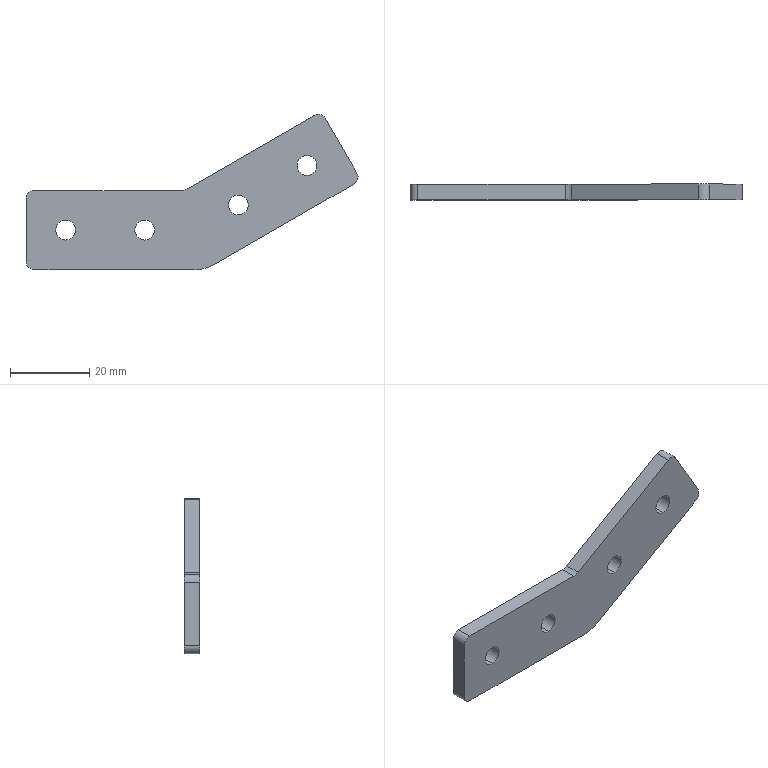Part | STEP file | 150-degree side frame | 1 solid | 22 faces | box 83.909 x 4 x 39.268 mm | volume 6499 mm3 | cylinder 14 | plane 8 | commonest cylinder face diameters 5 x8 4 x4 6 x1 20 x1